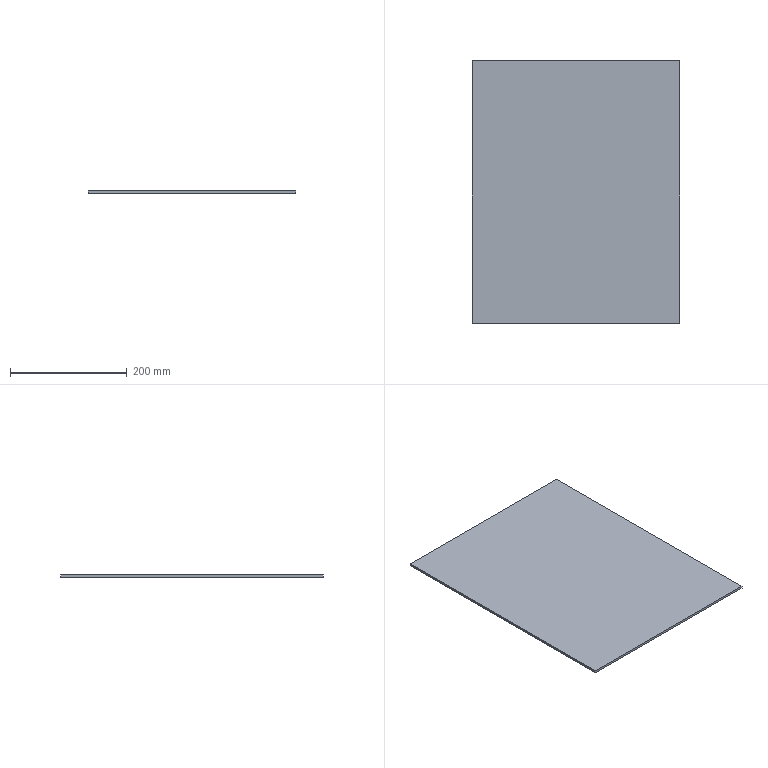Part | SolidWorks | features Extrusion 1 | 1 solid | 6 faces | box 356 x 450 x 4 mm | volume 640800 mm3 | plane 6
STEP:
#1=CARTESIAN_POINT('',(-178.,225.,0.));
#2=VERTEX_POINT('',#1);
#3=CARTESIAN_POINT('',(-178.,-225.,0.));
#4=VERTEX_POINT('',#3);
#5=CARTESIAN_POINT('',(-178.,-225.,0.));
#6=DIRECTION('',(0.,-1.,0.));
#7=VECTOR('',#6,1000.);
#8=LINE('',#5,#7);
#9=EDGE_CURVE('',#2,#4,#8,.T.);
#10=ORIENTED_EDGE('',*,*,#9,.T.);
#11=CARTESIAN_POINT('',(-178.,-225.,4.));
#12=VERTEX_POINT('',#11);
#13=CARTESIAN_POINT('',(-178.,-225.,4.));
#14=DIRECTION('',(0.,0.,-1.));
#15=VECTOR('',#14,1000.);
#16=LINE('',#13,#15);
#17=EDGE_CURVE('',#12,#4,#16,.T.);
#18=ORIENTED_EDGE('',*,*,#17,.F.);
#19=CARTESIAN_POINT('',(-178.,225.,4.));
#20=VERTEX_POINT('',#19);
#21=CARTESIAN_POINT('',(-178.,-225.,4.));
#22=DIRECTION('',(0.,-1.,0.));
#23=VECTOR('',#22,1000.);
#24=LINE('',#21,#23);
#25=EDGE_CURVE('',#20,#12,#24,.T.);
#26=ORIENTED_EDGE('',*,*,#25,.F.);
#27=CARTESIAN_POINT('',(-178.,225.,4.));
#28=DIRECTION('',(0.,0.,-1.));
#29=VECTOR('',#28,1000.);
#30=LINE('',#27,#29);
#31=EDGE_CURVE('',#20,#2,#30,.T.);
#32=ORIENTED_EDGE('',*,*,#31,.T.);
#33=EDGE_LOOP('',(#10,#18,#26,#32));
#34=FACE_OUTER_BOUND('',#33,.T.);
#35=CARTESIAN_POINT('',(-178.,-225.,4.));
#36=DIRECTION('',(1.,0.,0.));
#37=DIRECTION('',(0.,0.,-1.));
#38=AXIS2_PLACEMENT_3D('',#35,#36,#37);
#39=PLANE('',#38);
#40=ADVANCED_FACE('',(#34),#39,.F.);
#41=CARTESIAN_POINT('',(178.,-225.,0.));
#42=VERTEX_POINT('',#41);
#43=CARTESIAN_POINT('',(178.,-225.,0.));
#44=DIRECTION('',(1.,0.,0.));
#45=VECTOR('',#44,1000.);
#46=LINE('',#43,#45);
#47=EDGE_CURVE('',#4,#42,#46,.T.);
#48=ORIENTED_EDGE('',*,*,#47,.T.);
#49=CARTESIAN_POINT('',(178.,-225.,4.));
#50=VERTEX_POINT('',#49);
#51=CARTESIAN_POINT('',(178.,-225.,4.));
#52=DIRECTION('',(0.,0.,-1.));
#53=VECTOR('',#52,1000.);
#54=LINE('',#51,#53);
#55=EDGE_CURVE('',#50,#42,#54,.T.);
#56=ORIENTED_EDGE('',*,*,#55,.F.);
#57=CARTESIAN_POINT('',(178.,-225.,4.));
#58=DIRECTION('',(1.,0.,0.));
#59=VECTOR('',#58,1000.);
#60=LINE('',#57,#59);
#61=EDGE_CURVE('',#12,#50,#60,.T.);
#62=ORIENTED_EDGE('',*,*,#61,.F.);
#63=ORIENTED_EDGE('',*,*,#17,.T.);
#64=EDGE_LOOP('',(#48,#56,#62,#63));
#65=FACE_OUTER_BOUND('',#64,.T.);
#66=CARTESIAN_POINT('',(178.,-225.,4.));
#67=DIRECTION('',(0.,1.,0.));
#68=DIRECTION('',(-1.,0.,0.));
#69=AXIS2_PLACEMENT_3D('',#66,#67,#68);
#70=PLANE('',#69);
#71=ADVANCED_FACE('',(#65),#70,.F.);
#72=CARTESIAN_POINT('',(178.,225.,0.));
#73=VERTEX_POINT('',#72);
#74=CARTESIAN_POINT('',(178.,-225.,0.));
#75=DIRECTION('',(0.,1.,0.));
#76=VECTOR('',#75,1000.);
#77=LINE('',#74,#76);
#78=EDGE_CURVE('',#42,#73,#77,.T.);
#79=ORIENTED_EDGE('',*,*,#78,.T.);
#80=CARTESIAN_POINT('',(178.,225.,4.));
#81=VERTEX_POINT('',#80);
#82=CARTESIAN_POINT('',(178.,225.,4.));
#83=DIRECTION('',(0.,0.,-1.));
#84=VECTOR('',#83,1000.);
#85=LINE('',#82,#84);
#86=EDGE_CURVE('',#81,#73,#85,.T.);
#87=ORIENTED_EDGE('',*,*,#86,.F.);
#88=CARTESIAN_POINT('',(178.,-225.,4.));
#89=DIRECTION('',(0.,1.,0.));
#90=VECTOR('',#89,1000.);
#91=LINE('',#88,#90);
#92=EDGE_CURVE('',#50,#81,#91,.T.);
#93=ORIENTED_EDGE('',*,*,#92,.F.);
#94=ORIENTED_EDGE('',*,*,#55,.T.);
#95=EDGE_LOOP('',(#79,#87,#93,#94));
#96=FACE_OUTER_BOUND('',#95,.T.);
#97=CARTESIAN_POINT('',(178.,-225.,4.));
#98=DIRECTION('',(-1.,0.,0.));
#99=DIRECTION('',(0.,0.,1.));
#100=AXIS2_PLACEMENT_3D('',#97,#98,#99);
#101=PLANE('',#100);
#102=ADVANCED_FACE('',(#96),#101,.F.);
#103=CARTESIAN_POINT('',(178.,225.,0.));
#104=DIRECTION('',(-1.,0.,0.));
#105=VECTOR('',#104,1000.);
#106=LINE('',#103,#105);
#107=EDGE_CURVE('',#73,#2,#106,.T.);
#108=ORIENTED_EDGE('',*,*,#107,.T.);
#109=ORIENTED_EDGE('',*,*,#31,.F.);
#110=CARTESIAN_POINT('',(178.,225.,4.));
#111=DIRECTION('',(-1.,0.,0.));
#112=VECTOR('',#111,1000.);
#113=LINE('',#110,#112);
#114=EDGE_CURVE('',#81,#20,#113,.T.);
#115=ORIENTED_EDGE('',*,*,#114,.F.);
#116=ORIENTED_EDGE('',*,*,#86,.T.);
#117=EDGE_LOOP('',(#108,#109,#115,#116));
#118=FACE_OUTER_BOUND('',#117,.T.);
#119=CARTESIAN_POINT('',(178.,225.,4.));
#120=DIRECTION('',(0.,-1.,0.));
#121=DIRECTION('',(1.,0.,0.));
#122=AXIS2_PLACEMENT_3D('',#119,#120,#121);
#123=PLANE('',#122);
#124=ADVANCED_FACE('',(#118),#123,.F.);
#125=ORIENTED_EDGE('',*,*,#25,.T.);
#126=ORIENTED_EDGE('',*,*,#61,.T.);
#127=ORIENTED_EDGE('',*,*,#92,.T.);
#128=ORIENTED_EDGE('',*,*,#114,.T.);
#129=EDGE_LOOP('',(#125,#126,#127,#128));
#130=FACE_OUTER_BOUND('',#129,.T.);
#131=CARTESIAN_POINT('',(0.,0.,4.));
#132=DIRECTION('',(0.,0.,1.));
#133=DIRECTION('',(1.,0.,0.));
#134=AXIS2_PLACEMENT_3D('',#131,#132,#133);
#135=PLANE('',#134);
#136=ADVANCED_FACE('',(#130),#135,.T.);
#137=ORIENTED_EDGE('',*,*,#9,.F.);
#138=ORIENTED_EDGE('',*,*,#107,.F.);
#139=ORIENTED_EDGE('',*,*,#78,.F.);
#140=ORIENTED_EDGE('',*,*,#47,.F.);
#141=EDGE_LOOP('',(#137,#138,#139,#140));
#142=FACE_OUTER_BOUND('',#141,.T.);
#143=CARTESIAN_POINT('',(0.,0.,0.));
#144=DIRECTION('',(0.,0.,1.));
#145=DIRECTION('',(1.,0.,0.));
#146=AXIS2_PLACEMENT_3D('',#143,#144,#145);
#147=PLANE('',#146);
#148=ADVANCED_FACE('',(#142),#147,.F.);
#149=CLOSED_SHELL('',(#40,#71,#102,#124,#136,#148));
#150=MANIFOLD_SOLID_BREP('',#149);
#151=CARTESIAN_POINT('',(0.,0.,0.));
#152=DIRECTION('',(0.,0.,1.));
#153=DIRECTION('',(1.,0.,0.));
#154=AXIS2_PLACEMENT_3D('',#151,#152,#153);
#155=(LENGTH_UNIT()NAMED_UNIT(*)SI_UNIT(.MILLI.,.METRE.));
#156=UNCERTAINTY_MEASURE_WITH_UNIT(LENGTH_MEASURE(0.00001),#155,'','');
#157=(NAMED_UNIT(*)PLANE_ANGLE_UNIT()SI_UNIT($,.RADIAN.));
#158=(NAMED_UNIT(*)SI_UNIT($,.STERADIAN.)SOLID_ANGLE_UNIT());
#159=(GEOMETRIC_REPRESENTATION_CONTEXT(3)GLOBAL_UNCERTAINTY_ASSIGNED_CONTEXT((#156))GLOBAL_UNIT_ASSIGNED_CONTEXT((#155,#157,#158))REPRESENTATION_CONTEXT('',''));
#160=ADVANCED_BREP_SHAPE_REPRESENTATION('',(#150,#154),#159);